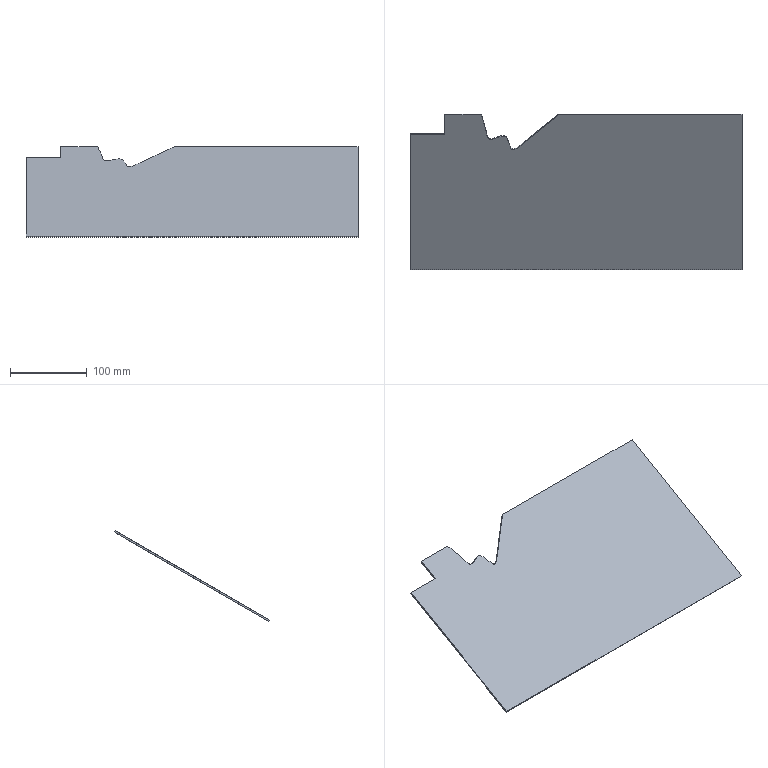Part | NX | features solid 2 | 1 solid | 11 faces | box 433.5 x 203.038 x 118.379 mm | volume 193522 mm3 | plane 9 | spline 2
STEP:
#1=CARTESIAN_POINT('',(-502.5,-191.,-72.946));
#2=VERTEX_POINT('',#1);
#3=CARTESIAN_POINT('',(-457.422,-191.,-72.946));
#4=VERTEX_POINT('',#3);
#5=CARTESIAN_POINT('',(-415.478,-191.,-72.946));
#6=DIRECTION('',(-1.,0.,0.));
#7=VECTOR('',#6,1000.);
#8=LINE('',#5,#7);
#9=EDGE_CURVE('',#2,#4,#8,.F.);
#10=ORIENTED_EDGE('',*,*,#9,.T.);
#11=CARTESIAN_POINT('',(-457.422,-190.,-74.678));
#12=VERTEX_POINT('',#11);
#13=CARTESIAN_POINT('',(-457.422,-140.,-161.281));
#14=DIRECTION('',(0.,-0.5,0.866));
#15=VECTOR('',#14,1000.);
#16=LINE('',#13,#15);
#17=EDGE_CURVE('',#12,#4,#16,.T.);
#18=ORIENTED_EDGE('',*,*,#17,.F.);
#19=CARTESIAN_POINT('',(-502.5,-190.,-74.678));
#20=VERTEX_POINT('',#19);
#21=CARTESIAN_POINT('',(-370.,-190.,-74.678));
#22=DIRECTION('',(1.,0.,0.));
#23=VECTOR('',#22,1000.);
#24=LINE('',#21,#23);
#25=EDGE_CURVE('',#20,#12,#24,.T.);
#26=ORIENTED_EDGE('',*,*,#25,.F.);
#27=CARTESIAN_POINT('',(-502.5,-97.191,-235.428));
#28=DIRECTION('',(0.,-0.5,0.866));
#29=VECTOR('',#28,1000.);
#30=LINE('',#27,#29);
#31=EDGE_CURVE('',#20,#2,#30,.T.);
#32=ORIENTED_EDGE('',*,*,#31,.T.);
#33=EDGE_LOOP('',(#10,#18,#26,#32));
#34=FACE_BOUND('',#33,.T.);
#35=CARTESIAN_POINT('',(-415.478,-140.,-161.281));
#36=DIRECTION('',(0.,-0.866,-0.5));
#37=DIRECTION('',(0.,0.5,-0.866));
#38=AXIS2_PLACEMENT_3D('',#35,#36,#37);
#39=PLANE('',#38);
#40=ADVANCED_FACE('',(#34),#39,.F.);
#41=CARTESIAN_POINT('',(-502.5,-367.603,-174.908));
#42=VERTEX_POINT('',#41);
#43=CARTESIAN_POINT('',(-502.5,-115.381,-29.287));
#44=DIRECTION('',(0.,-0.866,-0.5));
#45=VECTOR('',#44,1000.);
#46=LINE('',#43,#45);
#47=EDGE_CURVE('',#2,#42,#46,.T.);
#48=ORIENTED_EDGE('',*,*,#47,.F.);
#49=ORIENTED_EDGE('',*,*,#31,.F.);
#50=CARTESIAN_POINT('',(-502.5,-366.603,-176.64));
#51=VERTEX_POINT('',#50);
#52=CARTESIAN_POINT('',(-502.5,-114.381,-31.019));
#53=DIRECTION('',(0.,-0.866,-0.5));
#54=VECTOR('',#53,1000.);
#55=LINE('',#52,#54);
#56=EDGE_CURVE('',#20,#51,#55,.T.);
#57=ORIENTED_EDGE('',*,*,#56,.T.);
#58=CARTESIAN_POINT('',(-502.5,-273.793,-337.39));
#59=DIRECTION('',(0.,-0.5,0.866));
#60=VECTOR('',#59,1000.);
#61=LINE('',#58,#60);
#62=EDGE_CURVE('',#51,#42,#61,.T.);
#63=ORIENTED_EDGE('',*,*,#62,.T.);
#64=EDGE_LOOP('',(#48,#49,#57,#63));
#65=FACE_BOUND('',#64,.T.);
#66=CARTESIAN_POINT('',(-502.5,198.,-65.));
#67=DIRECTION('',(-1.,0.,0.));
#68=DIRECTION('',(0.,0.,-1.));
#69=AXIS2_PLACEMENT_3D('',#66,#67,#68);
#70=PLANE('',#69);
#71=ADVANCED_FACE('',(#65),#70,.T.);
#72=CARTESIAN_POINT('',(-69.,-367.603,-174.908));
#73=VERTEX_POINT('',#72);
#74=CARTESIAN_POINT('',(-370.,-367.603,-174.908));
#75=DIRECTION('',(1.,0.,0.));
#76=VECTOR('',#75,1000.);
#77=LINE('',#74,#76);
#78=EDGE_CURVE('',#42,#73,#77,.T.);
#79=ORIENTED_EDGE('',*,*,#78,.F.);
#80=ORIENTED_EDGE('',*,*,#62,.F.);
#81=CARTESIAN_POINT('',(-69.,-366.603,-176.64));
#82=VERTEX_POINT('',#81);
#83=CARTESIAN_POINT('',(-370.,-366.603,-176.64));
#84=DIRECTION('',(1.,0.,0.));
#85=VECTOR('',#84,1000.);
#86=LINE('',#83,#85);
#87=EDGE_CURVE('',#51,#82,#86,.T.);
#88=ORIENTED_EDGE('',*,*,#87,.T.);
#89=CARTESIAN_POINT('',(-69.,-318.851,-259.348));
#90=DIRECTION('',(0.,-0.5,0.866));
#91=VECTOR('',#90,1000.);
#92=LINE('',#89,#91);
#93=EDGE_CURVE('',#82,#73,#92,.T.);
#94=ORIENTED_EDGE('',*,*,#93,.T.);
#95=EDGE_LOOP('',(#79,#80,#88,#94));
#96=FACE_BOUND('',#95,.T.);
#97=CARTESIAN_POINT('',(-370.,-316.603,-263.242));
#98=DIRECTION('',(0.,-0.866,-0.5));
#99=DIRECTION('',(0.,0.5,-0.866));
#100=AXIS2_PLACEMENT_3D('',#97,#98,#99);
#101=PLANE('',#100);
#102=ADVANCED_FACE('',(#96),#101,.T.);
#103=CARTESIAN_POINT('',(-69.,-165.577,-58.268));
#104=VERTEX_POINT('',#103);
#105=CARTESIAN_POINT('',(-69.,-115.381,-29.287));
#106=DIRECTION('',(0.,-0.866,-0.5));
#107=VECTOR('',#106,1000.);
#108=LINE('',#105,#107);
#109=EDGE_CURVE('',#104,#73,#108,.T.);
#110=ORIENTED_EDGE('',*,*,#109,.T.);
#111=ORIENTED_EDGE('',*,*,#93,.F.);
#112=CARTESIAN_POINT('',(-69.,-164.577,-60.));
#113=VERTEX_POINT('',#112);
#114=CARTESIAN_POINT('',(-69.,-12.661,27.708));
#115=DIRECTION('',(0.,0.866,0.5));
#116=VECTOR('',#115,1000.);
#117=LINE('',#114,#116);
#118=EDGE_CURVE('',#82,#113,#117,.T.);
#119=ORIENTED_EDGE('',*,*,#118,.T.);
#120=CARTESIAN_POINT('',(-69.,-114.577,-146.603));
#121=DIRECTION('',(0.,-0.5,0.866));
#122=VECTOR('',#121,1000.);
#123=LINE('',#120,#122);
#124=EDGE_CURVE('',#113,#104,#123,.T.);
#125=ORIENTED_EDGE('',*,*,#124,.T.);
#126=EDGE_LOOP('',(#110,#111,#119,#125));
#127=FACE_BOUND('',#126,.T.);
#128=CARTESIAN_POINT('',(-69.,-64.381,-117.622));
#129=DIRECTION('',(-1.,0.,0.));
#130=DIRECTION('',(0.,0.,1.));
#131=AXIS2_PLACEMENT_3D('',#128,#129,#130);
#132=PLANE('',#131);
#133=ADVANCED_FACE('',(#127),#132,.F.);
#134=CARTESIAN_POINT('',(-308.051,-165.577,-58.268));
#135=VERTEX_POINT('',#134);
#136=CARTESIAN_POINT('',(-690.,-165.577,-58.268));
#137=DIRECTION('',(1.,0.,0.));
#138=VECTOR('',#137,1000.);
#139=LINE('',#136,#138);
#140=EDGE_CURVE('',#135,#104,#139,.T.);
#141=ORIENTED_EDGE('',*,*,#140,.T.);
#142=ORIENTED_EDGE('',*,*,#124,.F.);
#143=CARTESIAN_POINT('',(-308.051,-164.577,-60.));
#144=VERTEX_POINT('',#143);
#145=CARTESIAN_POINT('',(-370.,-164.577,-60.));
#146=DIRECTION('',(1.,0.,0.));
#147=VECTOR('',#146,1000.);
#148=LINE('',#145,#147);
#149=EDGE_CURVE('',#144,#113,#148,.T.);
#150=ORIENTED_EDGE('',*,*,#149,.F.);
#151=CARTESIAN_POINT('',(-308.051,-165.577,-58.268));
#152=CARTESIAN_POINT('',(-308.051,-165.243,-58.845));
#153=CARTESIAN_POINT('',(-308.051,-164.91,-59.423));
#154=CARTESIAN_POINT('',(-308.051,-164.577,-60.));
#155=B_SPLINE_CURVE_WITH_KNOTS('',3,(#151,#152,#153,#154),.UNSPECIFIED.,.F.,.F.,(4,4),(0.,0.01961),.UNSPECIFIED.);
#156=EDGE_CURVE('',#144,#135,#155,.F.);
#157=ORIENTED_EDGE('',*,*,#156,.T.);
#158=EDGE_LOOP('',(#141,#142,#150,#157));
#159=FACE_BOUND('',#158,.T.);
#160=CARTESIAN_POINT('',(-690.,-114.577,-146.603));
#161=DIRECTION('',(0.,-0.866,-0.5));
#162=DIRECTION('',(0.,0.5,-0.866));
#163=AXIS2_PLACEMENT_3D('',#160,#161,#162);
#164=PLANE('',#163);
#165=ADVANCED_FACE('',(#159),#164,.F.);
#166=CARTESIAN_POINT('',(-406.591,-174.699,-63.535));
#167=VERTEX_POINT('',#166);
#168=CARTESIAN_POINT('',(-308.051,-165.577,-58.268));
#169=CARTESIAN_POINT('',(-308.254,-165.738,-58.361));
#170=CARTESIAN_POINT('',(-309.078,-166.393,-58.739));
#171=CARTESIAN_POINT('',(-311.573,-168.377,-59.885));
#172=CARTESIAN_POINT('',(-314.699,-170.864,-61.32));
#173=CARTESIAN_POINT('',(-317.438,-173.043,-62.578));
#174=CARTESIAN_POINT('',(-319.159,-174.412,-63.369));
#175=CARTESIAN_POINT('',(-320.531,-175.504,-63.999));
#176=CARTESIAN_POINT('',(-321.734,-176.46,-64.552));
#177=CARTESIAN_POINT('',(-322.749,-177.268,-65.018));
#178=CARTESIAN_POINT('',(-323.368,-177.761,-65.302));
#179=CARTESIAN_POINT('',(-323.945,-178.22,-65.567));
#180=CARTESIAN_POINT('',(-324.267,-178.476,-65.715));
#181=CARTESIAN_POINT('',(-324.866,-178.952,-65.99));
#182=CARTESIAN_POINT('',(-326.005,-179.857,-66.513));
#183=CARTESIAN_POINT('',(-327.565,-181.096,-67.228));
#184=CARTESIAN_POINT('',(-329.008,-182.241,-67.889));
#185=CARTESIAN_POINT('',(-330.099,-183.104,-68.388));
#186=CARTESIAN_POINT('',(-330.751,-183.62,-68.685));
#187=CARTESIAN_POINT('',(-331.26,-184.023,-68.918));
#188=CARTESIAN_POINT('',(-331.563,-184.262,-69.056));
#189=CARTESIAN_POINT('',(-331.789,-184.44,-69.159));
#190=CARTESIAN_POINT('',(-331.889,-184.519,-69.204));
#191=CARTESIAN_POINT('',(-332.094,-184.681,-69.298));
#192=CARTESIAN_POINT('',(-332.422,-184.94,-69.447));
#193=CARTESIAN_POINT('',(-332.892,-185.311,-69.662));
#194=CARTESIAN_POINT('',(-333.473,-185.77,-69.927));
#195=CARTESIAN_POINT('',(-334.35,-186.462,-70.326));
#196=CARTESIAN_POINT('',(-335.768,-187.582,-70.972));
#197=CARTESIAN_POINT('',(-337.113,-188.645,-71.586));
#198=CARTESIAN_POINT('',(-338.186,-189.494,-72.076));
#199=CARTESIAN_POINT('',(-338.854,-190.023,-72.382));
#200=CARTESIAN_POINT('',(-339.296,-190.374,-72.584));
#201=CARTESIAN_POINT('',(-339.583,-190.601,-72.716));
#202=CARTESIAN_POINT('',(-339.731,-190.719,-72.784));
#203=CARTESIAN_POINT('',(-339.826,-190.794,-72.827));
#204=CARTESIAN_POINT('',(-339.867,-190.827,-72.846));
#205=CARTESIAN_POINT('',(-339.91,-190.862,-72.866));
#206=CARTESIAN_POINT('',(-339.899,-190.853,-72.861));
#207=CARTESIAN_POINT('',(-340.053,-190.976,-72.932));
#208=CARTESIAN_POINT('',(-340.29,-191.165,-73.041));
#209=CARTESIAN_POINT('',(-340.771,-191.55,-73.264));
#210=CARTESIAN_POINT('',(-341.409,-192.061,-73.558));
#211=CARTESIAN_POINT('',(-342.355,-192.817,-73.995));
#212=CARTESIAN_POINT('',(-343.384,-193.639,-74.47));
#213=CARTESIAN_POINT('',(-344.705,-194.696,-75.08));
#214=CARTESIAN_POINT('',(-345.431,-195.276,-75.415));
#215=CARTESIAN_POINT('',(-345.755,-195.535,-75.564));
#216=CARTESIAN_POINT('',(-345.829,-195.594,-75.598));
#217=CARTESIAN_POINT('',(-345.874,-195.63,-75.619));
#218=CARTESIAN_POINT('',(-345.862,-195.62,-75.614));
#219=CARTESIAN_POINT('',(-345.958,-195.696,-75.658));
#220=CARTESIAN_POINT('',(-346.164,-195.859,-75.751));
#221=CARTESIAN_POINT('',(-346.446,-196.081,-75.88));
#222=CARTESIAN_POINT('',(-346.815,-196.372,-76.048));
#223=CARTESIAN_POINT('',(-347.396,-196.83,-76.312));
#224=CARTESIAN_POINT('',(-348.418,-197.633,-76.776));
#225=CARTESIAN_POINT('',(-349.59,-198.549,-77.305));
#226=CARTESIAN_POINT('',(-350.61,-199.343,-77.763));
#227=CARTESIAN_POINT('',(-351.206,-199.806,-78.03));
#228=CARTESIAN_POINT('',(-351.55,-200.073,-78.184));
#229=CARTESIAN_POINT('',(-351.892,-200.337,-78.337));
#230=CARTESIAN_POINT('',(-351.989,-200.413,-78.381));
#231=CARTESIAN_POINT('',(-352.241,-200.61,-78.494));
#232=CARTESIAN_POINT('',(-352.844,-201.087,-78.77));
#233=CARTESIAN_POINT('',(-354.121,-202.108,-79.359));
#234=CARTESIAN_POINT('',(-355.859,-203.508,-80.167));
#235=CARTESIAN_POINT('',(-357.662,-204.965,-81.009));
#236=CARTESIAN_POINT('',(-358.887,-205.956,-81.581));
#237=CARTESIAN_POINT('',(-359.831,-206.715,-82.019));
#238=CARTESIAN_POINT('',(-360.359,-207.136,-82.262));
#239=CARTESIAN_POINT('',(-360.659,-207.374,-82.4));
#240=CARTESIAN_POINT('',(-360.752,-207.447,-82.442));
#241=CARTESIAN_POINT('',(-360.996,-207.639,-82.552));
#242=CARTESIAN_POINT('',(-361.347,-207.911,-82.709));
#243=CARTESIAN_POINT('',(-361.761,-208.225,-82.891));
#244=CARTESIAN_POINT('',(-362.402,-208.697,-83.164));
#245=CARTESIAN_POINT('',(-362.987,-209.108,-83.401));
#246=CARTESIAN_POINT('',(-363.56,-209.484,-83.618));
#247=CARTESIAN_POINT('',(-363.884,-209.689,-83.736));
#248=CARTESIAN_POINT('',(-364.508,-210.056,-83.948));
#249=CARTESIAN_POINT('',(-365.012,-210.321,-84.101));
#250=CARTESIAN_POINT('',(-365.536,-210.563,-84.241));
#251=CARTESIAN_POINT('',(-365.94,-210.729,-84.337));
#252=CARTESIAN_POINT('',(-366.646,-210.951,-84.465));
#253=CARTESIAN_POINT('',(-367.425,-211.082,-84.54));
#254=CARTESIAN_POINT('',(-368.333,-211.056,-84.525));
#255=CARTESIAN_POINT('',(-369.175,-210.699,-84.319));
#256=CARTESIAN_POINT('',(-369.765,-210.252,-84.061));
#257=CARTESIAN_POINT('',(-370.231,-209.75,-83.771));
#258=CARTESIAN_POINT('',(-370.469,-209.425,-83.584));
#259=CARTESIAN_POINT('',(-370.765,-208.98,-83.327));
#260=CARTESIAN_POINT('',(-371.03,-208.518,-83.06));
#261=CARTESIAN_POINT('',(-371.328,-207.923,-82.716));
#262=CARTESIAN_POINT('',(-371.493,-207.552,-82.502));
#263=CARTESIAN_POINT('',(-371.694,-207.072,-82.225));
#264=CARTESIAN_POINT('',(-371.857,-206.643,-81.978));
#265=CARTESIAN_POINT('',(-371.981,-206.302,-81.78));
#266=CARTESIAN_POINT('',(-372.097,-205.967,-81.587));
#267=CARTESIAN_POINT('',(-372.125,-205.885,-81.54));
#268=CARTESIAN_POINT('',(-372.208,-205.636,-81.396));
#269=CARTESIAN_POINT('',(-372.324,-205.28,-81.19));
#270=CARTESIAN_POINT('',(-372.501,-204.73,-80.873));
#271=CARTESIAN_POINT('',(-372.805,-203.771,-80.319));
#272=CARTESIAN_POINT('',(-373.133,-202.746,-79.727));
#273=CARTESIAN_POINT('',(-373.491,-201.665,-79.104));
#274=CARTESIAN_POINT('',(-373.753,-200.907,-78.666));
#275=CARTESIAN_POINT('',(-373.91,-200.471,-78.414));
#276=CARTESIAN_POINT('',(-374.005,-200.214,-78.266));
#277=CARTESIAN_POINT('',(-374.041,-200.116,-78.209));
#278=CARTESIAN_POINT('',(-374.198,-199.709,-77.974));
#279=CARTESIAN_POINT('',(-374.37,-199.289,-77.732));
#280=CARTESIAN_POINT('',(-374.697,-198.534,-77.296));
#281=CARTESIAN_POINT('',(-375.179,-197.571,-76.74));
#282=CARTESIAN_POINT('',(-375.8,-196.546,-76.148));
#283=CARTESIAN_POINT('',(-376.679,-195.372,-75.47));
#284=CARTESIAN_POINT('',(-377.626,-194.484,-74.958));
#285=CARTESIAN_POINT('',(-378.676,-193.875,-74.606));
#286=CARTESIAN_POINT('',(-379.431,-193.577,-74.434));
#287=CARTESIAN_POINT('',(-380.497,-193.358,-74.308));
#288=CARTESIAN_POINT('',(-381.613,-193.318,-74.284));
#289=CARTESIAN_POINT('',(-382.632,-193.409,-74.337));
#290=CARTESIAN_POINT('',(-383.405,-193.546,-74.416));
#291=CARTESIAN_POINT('',(-383.833,-193.637,-74.469));
#292=CARTESIAN_POINT('',(-384.236,-193.735,-74.525));
#293=CARTESIAN_POINT('',(-384.354,-193.767,-74.544));
#294=CARTESIAN_POINT('',(-384.633,-193.843,-74.588));
#295=CARTESIAN_POINT('',(-385.117,-193.986,-74.67));
#296=CARTESIAN_POINT('',(-386.299,-194.367,-74.89));
#297=CARTESIAN_POINT('',(-388.071,-195.014,-75.264));
#298=CARTESIAN_POINT('',(-390.198,-195.816,-75.727));
#299=CARTESIAN_POINT('',(-391.407,-196.255,-75.98));
#300=CARTESIAN_POINT('',(-392.231,-196.542,-76.146));
#301=CARTESIAN_POINT('',(-392.665,-196.686,-76.229));
#302=CARTESIAN_POINT('',(-392.914,-196.765,-76.274));
#303=CARTESIAN_POINT('',(-392.99,-196.789,-76.288));
#304=CARTESIAN_POINT('',(-393.407,-196.911,-76.359));
#305=CARTESIAN_POINT('',(-393.833,-197.025,-76.425));
#306=CARTESIAN_POINT('',(-394.611,-197.212,-76.533));
#307=CARTESIAN_POINT('',(-395.626,-197.383,-76.632));
#308=CARTESIAN_POINT('',(-396.547,-197.445,-76.667));
#309=CARTESIAN_POINT('',(-397.253,-197.42,-76.652));
#310=CARTESIAN_POINT('',(-397.683,-197.38,-76.63));
#311=CARTESIAN_POINT('',(-398.358,-197.252,-76.555));
#312=CARTESIAN_POINT('',(-399.085,-197.013,-76.417));
#313=CARTESIAN_POINT('',(-399.923,-196.538,-76.144));
#314=CARTESIAN_POINT('',(-400.501,-195.946,-75.802));
#315=CARTESIAN_POINT('',(-400.934,-195.365,-75.466));
#316=CARTESIAN_POINT('',(-401.27,-194.783,-75.13));
#317=CARTESIAN_POINT('',(-401.416,-194.48,-74.955));
#318=CARTESIAN_POINT('',(-401.666,-193.917,-74.63));
#319=CARTESIAN_POINT('',(-401.937,-193.158,-74.192));
#320=CARTESIAN_POINT('',(-402.192,-192.271,-73.68));
#321=CARTESIAN_POINT('',(-402.359,-191.576,-73.278));
#322=CARTESIAN_POINT('',(-402.446,-191.182,-73.051));
#323=CARTESIAN_POINT('',(-402.522,-190.815,-72.839));
#324=CARTESIAN_POINT('',(-402.549,-190.678,-72.76));
#325=CARTESIAN_POINT('',(-402.606,-190.384,-72.59));
#326=CARTESIAN_POINT('',(-402.706,-189.844,-72.279));
#327=CARTESIAN_POINT('',(-402.842,-189.052,-71.821));
#328=CARTESIAN_POINT('',(-402.997,-188.128,-71.288));
#329=CARTESIAN_POINT('',(-403.092,-187.575,-70.968));
#330=CARTESIAN_POINT('',(-403.157,-187.194,-70.749));
#331=CARTESIAN_POINT('',(-403.205,-186.92,-70.59));
#332=CARTESIAN_POINT('',(-403.227,-186.796,-70.519));
#333=CARTESIAN_POINT('',(-403.285,-186.475,-70.333));
#334=CARTESIAN_POINT('',(-403.35,-186.12,-70.129));
#335=CARTESIAN_POINT('',(-403.473,-185.48,-69.759));
#336=CARTESIAN_POINT('',(-403.65,-184.615,-69.26));
#337=CARTESIAN_POINT('',(-403.873,-183.626,-68.688));
#338=CARTESIAN_POINT('',(-404.106,-182.688,-68.147));
#339=CARTESIAN_POINT('',(-404.342,-181.82,-67.646));
#340=CARTESIAN_POINT('',(-404.626,-180.842,-67.081));
#341=CARTESIAN_POINT('',(-404.889,-179.989,-66.589));
#342=CARTESIAN_POINT('',(-405.126,-179.246,-66.16));
#343=CARTESIAN_POINT('',(-405.292,-178.738,-65.867));
#344=CARTESIAN_POINT('',(-405.55,-177.956,-65.415));
#345=CARTESIAN_POINT('',(-405.826,-177.112,-64.928));
#346=CARTESIAN_POINT('',(-406.254,-175.791,-64.165));
#347=CARTESIAN_POINT('',(-406.489,-175.042,-63.732));
#348=CARTESIAN_POINT('',(-406.591,-174.699,-63.535));
#349=B_SPLINE_CURVE_WITH_KNOTS('',3,(#168,#169,#170,#171,#172,#173,#174,#175,#176,#177,#178,#179,#180,#181,#182,#183,#184,#185,#186,#187,#188,#189,#190,#191,#192,#193,#194,#195,#196,#197,#198,#199,#200,#201,#202,#203,#204,#205,#206,#207,#208,#209,#210,#211,#212,#213,#214,#215,#216,#217,#218,#219,#220,#221,#222,#223,#224,#225,#226,#227,#228,#229,#230,#231,#232,#233,#234,#235,#236,#237,#238,#239,#240,#241,#242,#243,#244,#245,#246,#247,#248,#249,#250,#251,#252,#253,#254,#255,#256,#257,#258,#259,#260,#261,#262,#263,#264,#265,#266,#267,#268,#269,#270,#271,#272,#273,#274,#275,#276,#277,#278,#279,#280,#281,#282,#283,#284,#285,#286,#287,#288,#289,#290,#291,#292,#293,#294,#295,#296,#297,#298,#299,#300,#301,#302,#303,#304,#305,#306,#307,#308,#309,#310,#311,#312,#313,#314,#315,#316,#317,#318,#319,#320,#321,#322,#323,#324,#325,#326,#327,#328,#329,#330,#331,#332,#333,#334,#335,#336,#337,#338,#339,#340,#341,#342,#343,#344,#345,#346,#347,#348),.UNSPECIFIED.,.F.,.F.,(4,1,1,1,1,1,1,1,1,1,1,1,1,1,1,1,1,1,1,1,1,1,1,1,1,1,1,1,1,1,1,1,1,1,1,1,1,1,1,1,1,1,1,1,1,1,1,1,1,1,1,1,1,1,1,1,1,1,1,1,1,1,1,1,1,1,1,1,1,1,1,1,1,1,1,1,1,1,1,1,1,1,1,1,1,1,1,1,1,1,1,1,1,1,1,1,1,1,1,1,1,1,1,1,1,1,1,1,1,1,1,1,1,1,1,1,1,1,1,1,1,1,1,1,1,1,1,1,1,1,1,1,1,1,1,1,1,1,1,1,1,1,1,1,1,1,1,1,1,1,1,1,1,1,1,1,1,1,1,1,1,1,1,1,1,1,1,1,1,1,1,1,1,1,1,1,1,1,4),(0.,0.03125,0.0625,0.09375,0.1094,0.1172,0.125,0.1328,0.1367,0.1406,0.1426,0.1445,0.1484,0.1562,0.1719,0.1875,0.1953,0.2031,0.207,0.2109,0.2129,0.2139,0.2148,0.2168,0.2188,0.2227,0.2266,0.2344,0.25,0.2578,0.2656,0.2734,0.2773,0.2812,0.2832,0.2842,0.2852,0.2856,0.2861,0.2871,0.2891,0.293,0.2969,0.3047,0.3125,0.3281,0.332,0.3359,0.3379,0.3389,0.3398,0.3418,0.3438,0.3477,0.3516,0.3594,0.375,0.3828,0.3867,0.3906,0.3926,0.3945,0.3984,0.4062,0.4219,0.4375,0.4453,0.4531,0.4609,0.4688,0.4707,0.4727,0.4746,0.4766,0.4805,0.4844,0.4922,0.4961,0.5,0.5039,0.5078,0.5117,0.5156,0.5195,0.5234,0.5312,0.5391,0.543,0.5469,0.5508,0.5547,0.5586,0.5625,0.5664,0.5703,0.5742,0.5762,0.5781,0.5801,0.582,0.5859,0.5898,0.5938,0.6016,0.6094,0.6172,0.6211,0.623,0.625,0.627,0.6289,0.6328,0.6406,0.6484,0.6562,0.6719,0.6797,0.6875,0.6953,0.7031,0.7109,0.7148,0.7168,0.7188,0.7207,0.7227,0.7266,0.7344,0.75,0.7578,0.7656,0.7734,0.7773,0.7793,0.7812,0.7832,0.7852,0.7891,0.7969,0.8047,0.8086,0.8125,0.8164,0.8203,0.8281,0.8359,0.8398,0.8438,0.8477,0.8516,0.8594,0.8672,0.8711,0.873,0.875,0.877,0.8789,0.8828,0.8906,0.8945,0.8984,0.9023,0.9043,0.9062,0.9082,0.9102,0.9141,0.9219,0.9297,0.9375,0.9453,0.9531,0.9609,0.9648,0.9688,0.9727,0.9766,0.9844,1.),.UNSPECIFIED.);
#350=EDGE_CURVE('',#167,#135,#349,.F.);
#351=ORIENTED_EDGE('',*,*,#350,.T.);
#352=ORIENTED_EDGE('',*,*,#156,.F.);
#353=CARTESIAN_POINT('',(-406.591,-173.699,-65.267));
#354=VERTEX_POINT('',#353);
#355=CARTESIAN_POINT('',(-406.591,-173.699,-65.267));
#356=CARTESIAN_POINT('',(-406.198,-175.018,-66.028));
#357=CARTESIAN_POINT('',(-405.31,-177.635,-67.539));
#358=CARTESIAN_POINT('',(-404.07,-181.579,-69.816));
#359=CARTESIAN_POINT('',(-403.218,-185.599,-72.137));
#360=CARTESIAN_POINT('',(-402.724,-188.984,-74.092));
#361=CARTESIAN_POINT('',(-402.116,-191.664,-75.639));
#362=CARTESIAN_POINT('',(-401.443,-193.608,-76.761));
#363=CARTESIAN_POINT('',(-400.277,-195.451,-77.825));
#364=CARTESIAN_POINT('',(-398.119,-196.479,-78.419));
#365=CARTESIAN_POINT('',(-395.713,-196.453,-78.404));
#366=CARTESIAN_POINT('',(-393.422,-195.965,-78.122));
#367=CARTESIAN_POINT('',(-391.237,-195.199,-77.68));
#368=CARTESIAN_POINT('',(-389.076,-194.396,-77.216));
#369=CARTESIAN_POINT('',(-386.916,-193.585,-76.748));
#370=CARTESIAN_POINT('',(-384.735,-192.829,-76.311));
#371=CARTESIAN_POINT('',(-382.478,-192.321,-76.018));
#372=CARTESIAN_POINT('',(-380.027,-192.293,-76.002));
#373=CARTESIAN_POINT('',(-377.81,-193.228,-76.542));
#374=CARTESIAN_POINT('',(-376.246,-194.838,-77.471));
#375=CARTESIAN_POINT('',(-375.094,-196.659,-78.523));
#376=CARTESIAN_POINT('',(-373.938,-199.203,-79.991));
#377=CARTESIAN_POINT('',(-373.091,-201.861,-81.526));
#378=CARTESIAN_POINT('',(-372.258,-204.517,-83.06));
#379=CARTESIAN_POINT('',(-371.569,-206.489,-84.198));
#380=CARTESIAN_POINT('',(-370.763,-208.085,-85.12));
#381=CARTESIAN_POINT('',(-369.85,-209.221,-85.775));
#382=CARTESIAN_POINT('',(-368.903,-209.888,-86.16));
#383=CARTESIAN_POINT('',(-367.701,-210.131,-86.301));
#384=CARTESIAN_POINT('',(-366.103,-209.875,-86.153));
#385=CARTESIAN_POINT('',(-364.359,-209.024,-85.662));
#386=CARTESIAN_POINT('',(-362.466,-207.771,-84.938));
#387=CARTESIAN_POINT('',(-360.088,-205.946,-83.884));
#388=CARTESIAN_POINT('',(-357.201,-203.588,-82.523));
#389=CARTESIAN_POINT('',(-353.721,-200.772,-80.897));
#390=CARTESIAN_POINT('',(-350.184,-198.011,-79.303));
#391=CARTESIAN_POINT('',(-346.645,-195.251,-77.71));
#392=CARTESIAN_POINT('',(-341.984,-191.516,-75.553));
#393=CARTESIAN_POINT('',(-336.139,-186.866,-72.869));
#394=CARTESIAN_POINT('',(-329.092,-181.318,-69.665));
#395=CARTESIAN_POINT('',(-322.081,-175.735,-66.442));
#396=CARTESIAN_POINT('',(-315.065,-170.157,-63.221));
#397=CARTESIAN_POINT('',(-310.391,-166.435,-61.073));
#398=CARTESIAN_POINT('',(-308.051,-164.577,-60.));
#399=B_SPLINE_CURVE_WITH_KNOTS('',3,(#355,#356,#357,#358,#359,#360,#361,#362,#363,#364,#365,#366,#367,#368,#369,#370,#371,#372,#373,#374,#375,#376,#377,#378,#379,#380,#381,#382,#383,#384,#385,#386,#387,#388,#389,#390,#391,#392,#393,#394,#395,#396,#397,#398),.UNSPECIFIED.,.F.,.F.,(4,1,1,1,1,1,1,1,1,1,1,1,1,1,1,1,1,1,1,1,1,1,1,1,1,1,1,1,1,1,1,1,1,1,1,1,1,1,1,1,1,4),(0.,0.004714,0.009429,0.01414,0.01886,0.02121,0.02357,0.02593,0.02829,0.03064,0.033,0.03536,0.03771,0.04007,0.04243,0.04479,0.04714,0.0495,0.05186,0.05422,0.05657,0.06129,0.06364,0.066,0.06836,0.06954,0.07072,0.07189,0.07307,0.07543,0.07779,0.08014,0.08486,0.08957,0.09429,0.099,0.1037,0.1131,0.1226,0.132,0.1414,0.1509),.UNSPECIFIED.);
#400=EDGE_CURVE('',#354,#144,#399,.T.);
#401=ORIENTED_EDGE('',*,*,#400,.F.);
#402=CARTESIAN_POINT('',(-406.591,-174.699,-63.535));
#403=CARTESIAN_POINT('',(-406.591,-174.366,-64.112));
#404=CARTESIAN_POINT('',(-406.591,-174.033,-64.689));
#405=CARTESIAN_POINT('',(-406.591,-173.699,-65.267));
#406=B_SPLINE_CURVE_WITH_KNOTS('',3,(#402,#403,#404,#405),.UNSPECIFIED.,.F.,.F.,(4,4),(0.,0.01961),.UNSPECIFIED.);
#407=EDGE_CURVE('',#354,#167,#406,.F.);
#408=ORIENTED_EDGE('',*,*,#407,.T.);
#409=EDGE_LOOP('',(#351,#352,#401,#408));
#410=FACE_BOUND('',#409,.T.);
#411=CARTESIAN_POINT('',(-308.051,-164.577,-60.));
#412=CARTESIAN_POINT('',(-308.051,-165.577,-58.268));
#413=CARTESIAN_POINT('',(-308.254,-164.738,-60.093));
#414=CARTESIAN_POINT('',(-308.254,-165.738,-58.361));
#415=CARTESIAN_POINT('',(-309.078,-165.393,-60.471));
#416=CARTESIAN_POINT('',(-309.078,-166.393,-58.739));
#417=CARTESIAN_POINT('',(-311.573,-167.377,-61.617));
#418=CARTESIAN_POINT('',(-311.573,-168.377,-59.885));
#419=CARTESIAN_POINT('',(-314.699,-169.864,-63.052));
#420=CARTESIAN_POINT('',(-314.699,-170.864,-61.32));
#421=CARTESIAN_POINT('',(-317.438,-172.043,-64.31));
#422=CARTESIAN_POINT('',(-317.438,-173.043,-62.578));
#423=CARTESIAN_POINT('',(-319.159,-173.412,-65.101));
#424=CARTESIAN_POINT('',(-319.159,-174.412,-63.369));
#425=CARTESIAN_POINT('',(-320.531,-174.504,-65.731));
#426=CARTESIAN_POINT('',(-320.531,-175.504,-63.999));
#427=CARTESIAN_POINT('',(-321.734,-175.46,-66.284));
#428=CARTESIAN_POINT('',(-321.734,-176.46,-64.552));
#429=CARTESIAN_POINT('',(-322.749,-176.268,-66.75));
#430=CARTESIAN_POINT('',(-322.749,-177.268,-65.018));
#431=CARTESIAN_POINT('',(-323.368,-176.761,-67.034));
#432=CARTESIAN_POINT('',(-323.368,-177.761,-65.302));
#433=CARTESIAN_POINT('',(-323.945,-177.22,-67.299));
#434=CARTESIAN_POINT('',(-323.945,-178.22,-65.567));
#435=CARTESIAN_POINT('',(-324.267,-177.476,-67.447));
#436=CARTESIAN_POINT('',(-324.267,-178.476,-65.715));
#437=CARTESIAN_POINT('',(-324.866,-177.952,-67.722));
#438=CARTESIAN_POINT('',(-324.866,-178.952,-65.99));
#439=CARTESIAN_POINT('',(-326.005,-178.857,-68.245));
#440=CARTESIAN_POINT('',(-326.005,-179.857,-66.513));
#441=CARTESIAN_POINT('',(-327.565,-180.096,-68.96));
#442=CARTESIAN_POINT('',(-327.565,-181.096,-67.228));
#443=CARTESIAN_POINT('',(-329.008,-181.241,-69.621));
#444=CARTESIAN_POINT('',(-329.008,-182.241,-67.889));
#445=CARTESIAN_POINT('',(-330.099,-182.104,-70.12));
#446=CARTESIAN_POINT('',(-330.099,-183.104,-68.388));
#447=CARTESIAN_POINT('',(-330.751,-182.62,-70.417));
#448=CARTESIAN_POINT('',(-330.751,-183.62,-68.685));
#449=CARTESIAN_POINT('',(-331.26,-183.023,-70.65));
#450=CARTESIAN_POINT('',(-331.26,-184.023,-68.918));
#451=CARTESIAN_POINT('',(-331.563,-183.262,-70.788));
#452=CARTESIAN_POINT('',(-331.563,-184.262,-69.056));
#453=CARTESIAN_POINT('',(-331.789,-183.44,-70.891));
#454=CARTESIAN_POINT('',(-331.789,-184.44,-69.159));
#455=CARTESIAN_POINT('',(-331.889,-183.519,-70.936));
#456=CARTESIAN_POINT('',(-331.889,-184.519,-69.204));
#457=CARTESIAN_POINT('',(-332.094,-183.681,-71.03));
#458=CARTESIAN_POINT('',(-332.094,-184.681,-69.298));
#459=CARTESIAN_POINT('',(-332.422,-183.94,-71.179));
#460=CARTESIAN_POINT('',(-332.422,-184.94,-69.447));
#461=CARTESIAN_POINT('',(-332.892,-184.311,-71.394));
#462=CARTESIAN_POINT('',(-332.892,-185.311,-69.662));
#463=CARTESIAN_POINT('',(-333.473,-184.77,-71.659));
#464=CARTESIAN_POINT('',(-333.473,-185.77,-69.927));
#465=CARTESIAN_POINT('',(-334.35,-185.462,-72.058));
#466=CARTESIAN_POINT('',(-334.35,-186.462,-70.326));
#467=CARTESIAN_POINT('',(-335.768,-186.582,-72.705));
#468=CARTESIAN_POINT('',(-335.768,-187.582,-70.972));
#469=CARTESIAN_POINT('',(-337.113,-187.645,-73.318));
#470=CARTESIAN_POINT('',(-337.113,-188.645,-71.586));
#471=CARTESIAN_POINT('',(-338.186,-188.494,-73.808));
#472=CARTESIAN_POINT('',(-338.186,-189.494,-72.076));
#473=CARTESIAN_POINT('',(-338.854,-189.023,-74.114));
#474=CARTESIAN_POINT('',(-338.854,-190.023,-72.382));
#475=CARTESIAN_POINT('',(-339.296,-189.374,-74.316));
#476=CARTESIAN_POINT('',(-339.296,-190.374,-72.584));
#477=CARTESIAN_POINT('',(-339.583,-189.601,-74.448));
#478=CARTESIAN_POINT('',(-339.583,-190.601,-72.716));
#479=CARTESIAN_POINT('',(-339.731,-189.719,-74.516));
#480=CARTESIAN_POINT('',(-339.731,-190.719,-72.784));
#481=CARTESIAN_POINT('',(-339.826,-189.794,-74.559));
#482=CARTESIAN_POINT('',(-339.826,-190.794,-72.827));
#483=CARTESIAN_POINT('',(-339.867,-189.827,-74.578));
#484=CARTESIAN_POINT('',(-339.867,-190.827,-72.846));
#485=CARTESIAN_POINT('',(-339.91,-189.862,-74.598));
#486=CARTESIAN_POINT('',(-339.91,-190.862,-72.866));
#487=CARTESIAN_POINT('',(-339.899,-189.853,-74.593));
#488=CARTESIAN_POINT('',(-339.899,-190.853,-72.861));
#489=CARTESIAN_POINT('',(-340.053,-189.976,-74.664));
#490=CARTESIAN_POINT('',(-340.053,-190.976,-72.932));
#491=CARTESIAN_POINT('',(-340.29,-190.165,-74.774));
#492=CARTESIAN_POINT('',(-340.29,-191.165,-73.041));
#493=CARTESIAN_POINT('',(-340.771,-190.55,-74.996));
#494=CARTESIAN_POINT('',(-340.771,-191.55,-73.264));
#495=CARTESIAN_POINT('',(-341.409,-191.061,-75.29));
#496=CARTESIAN_POINT('',(-341.409,-192.061,-73.558));
#497=CARTESIAN_POINT('',(-342.355,-191.817,-75.727));
#498=CARTESIAN_POINT('',(-342.355,-192.817,-73.995));
#499=CARTESIAN_POINT('',(-343.384,-192.639,-76.202));
#500=CARTESIAN_POINT('',(-343.384,-193.639,-74.47));
#501=CARTESIAN_POINT('',(-344.705,-193.696,-76.812));
#502=CARTESIAN_POINT('',(-344.705,-194.696,-75.08));
#503=CARTESIAN_POINT('',(-345.431,-194.276,-77.147));
#504=CARTESIAN_POINT('',(-345.431,-195.276,-75.415));
#505=CARTESIAN_POINT('',(-345.755,-194.535,-77.296));
#506=CARTESIAN_POINT('',(-345.755,-195.535,-75.564));
#507=CARTESIAN_POINT('',(-345.829,-194.594,-77.331));
#508=CARTESIAN_POINT('',(-345.829,-195.594,-75.598));
#509=CARTESIAN_POINT('',(-345.874,-194.63,-77.351));
#510=CARTESIAN_POINT('',(-345.874,-195.63,-75.619));
#511=CARTESIAN_POINT('',(-345.862,-194.62,-77.346));
#512=CARTESIAN_POINT('',(-345.862,-195.62,-75.614));
#513=CARTESIAN_POINT('',(-345.958,-194.696,-77.39));
#514=CARTESIAN_POINT('',(-345.958,-195.696,-75.658));
#515=CARTESIAN_POINT('',(-346.164,-194.859,-77.483));
#516=CARTESIAN_POINT('',(-346.164,-195.859,-75.751));
#517=CARTESIAN_POINT('',(-346.446,-195.081,-77.612));
#518=CARTESIAN_POINT('',(-346.446,-196.081,-75.88));
#519=CARTESIAN_POINT('',(-346.815,-195.372,-77.78));
#520=CARTESIAN_POINT('',(-346.815,-196.372,-76.048));
#521=CARTESIAN_POINT('',(-347.396,-195.83,-78.044));
#522=CARTESIAN_POINT('',(-347.396,-196.83,-76.312));
#523=CARTESIAN_POINT('',(-348.418,-196.633,-78.508));
#524=CARTESIAN_POINT('',(-348.418,-197.633,-76.776));
#525=CARTESIAN_POINT('',(-349.59,-197.549,-79.037));
#526=CARTESIAN_POINT('',(-349.59,-198.549,-77.305));
#527=CARTESIAN_POINT('',(-350.61,-198.343,-79.495));
#528=CARTESIAN_POINT('',(-350.61,-199.343,-77.763));
#529=CARTESIAN_POINT('',(-351.206,-198.806,-79.762));
#530=CARTESIAN_POINT('',(-351.206,-199.806,-78.03));
#531=CARTESIAN_POINT('',(-351.55,-199.073,-79.916));
#532=CARTESIAN_POINT('',(-351.55,-200.073,-78.184));
#533=CARTESIAN_POINT('',(-351.892,-199.337,-80.069));
#534=CARTESIAN_POINT('',(-351.892,-200.337,-78.337));
#535=CARTESIAN_POINT('',(-351.989,-199.413,-80.113));
#536=CARTESIAN_POINT('',(-351.989,-200.413,-78.381));
#537=CARTESIAN_POINT('',(-352.241,-199.61,-80.226));
#538=CARTESIAN_POINT('',(-352.241,-200.61,-78.494));
#539=CARTESIAN_POINT('',(-352.844,-200.087,-80.502));
#540=CARTESIAN_POINT('',(-352.844,-201.087,-78.77));
#541=CARTESIAN_POINT('',(-354.121,-201.108,-81.091));
#542=CARTESIAN_POINT('',(-354.121,-202.108,-79.359));
#543=CARTESIAN_POINT('',(-355.859,-202.508,-81.899));
#544=CARTESIAN_POINT('',(-355.859,-203.508,-80.167));
#545=CARTESIAN_POINT('',(-357.662,-203.965,-82.741));
#546=CARTESIAN_POINT('',(-357.662,-204.965,-81.009));
#547=CARTESIAN_POINT('',(-358.887,-204.956,-83.313));
#548=CARTESIAN_POINT('',(-358.887,-205.956,-81.581));
#549=CARTESIAN_POINT('',(-359.831,-205.715,-83.751));
#550=CARTESIAN_POINT('',(-359.831,-206.715,-82.019));
#551=CARTESIAN_POINT('',(-360.359,-206.136,-83.994));
#552=CARTESIAN_POINT('',(-360.359,-207.136,-82.262));
#553=CARTESIAN_POINT('',(-360.659,-206.374,-84.132));
#554=CARTESIAN_POINT('',(-360.659,-207.374,-82.4));
#555=CARTESIAN_POINT('',(-360.752,-206.447,-84.174));
#556=CARTESIAN_POINT('',(-360.752,-207.447,-82.442));
#557=CARTESIAN_POINT('',(-360.996,-206.639,-84.284));
#558=CARTESIAN_POINT('',(-360.996,-207.639,-82.552));
#559=CARTESIAN_POINT('',(-361.347,-206.911,-84.441));
#560=CARTESIAN_POINT('',(-361.347,-207.911,-82.709));
#561=CARTESIAN_POINT('',(-361.761,-207.225,-84.623));
#562=CARTESIAN_POINT('',(-361.761,-208.225,-82.891));
#563=CARTESIAN_POINT('',(-362.402,-207.697,-84.896));
#564=CARTESIAN_POINT('',(-362.402,-208.697,-83.164));
#565=CARTESIAN_POINT('',(-362.987,-208.108,-85.133));
#566=CARTESIAN_POINT('',(-362.987,-209.108,-83.401));
#567=CARTESIAN_POINT('',(-363.56,-208.484,-85.35));
#568=CARTESIAN_POINT('',(-363.56,-209.484,-83.618));
#569=CARTESIAN_POINT('',(-363.884,-208.689,-85.468));
#570=CARTESIAN_POINT('',(-363.884,-209.689,-83.736));
#571=CARTESIAN_POINT('',(-364.508,-209.056,-85.68));
#572=CARTESIAN_POINT('',(-364.508,-210.056,-83.948));
#573=CARTESIAN_POINT('',(-365.012,-209.321,-85.833));
#574=CARTESIAN_POINT('',(-365.012,-210.321,-84.101));
#575=CARTESIAN_POINT('',(-365.536,-209.563,-85.973));
#576=CARTESIAN_POINT('',(-365.536,-210.563,-84.241));
#577=CARTESIAN_POINT('',(-365.94,-209.729,-86.069));
#578=CARTESIAN_POINT('',(-365.94,-210.729,-84.337));
#579=CARTESIAN_POINT('',(-366.646,-209.951,-86.197));
#580=CARTESIAN_POINT('',(-366.646,-210.951,-84.465));
#581=CARTESIAN_POINT('',(-367.425,-210.082,-86.272));
#582=CARTESIAN_POINT('',(-367.425,-211.082,-84.54));
#583=CARTESIAN_POINT('',(-368.333,-210.056,-86.257));
#584=CARTESIAN_POINT('',(-368.333,-211.056,-84.525));
#585=CARTESIAN_POINT('',(-369.175,-209.699,-86.051));
#586=CARTESIAN_POINT('',(-369.175,-210.699,-84.319));
#587=CARTESIAN_POINT('',(-369.765,-209.252,-85.793));
#588=CARTESIAN_POINT('',(-369.765,-210.252,-84.061));
#589=CARTESIAN_POINT('',(-370.231,-208.75,-85.503));
#590=CARTESIAN_POINT('',(-370.231,-209.75,-83.771));
#591=CARTESIAN_POINT('',(-370.469,-208.425,-85.316));
#592=CARTESIAN_POINT('',(-370.469,-209.425,-83.584));
#593=CARTESIAN_POINT('',(-370.765,-207.98,-85.059));
#594=CARTESIAN_POINT('',(-370.765,-208.98,-83.327));
#595=CARTESIAN_POINT('',(-371.03,-207.518,-84.792));
#596=CARTESIAN_POINT('',(-371.03,-208.518,-83.06));
#597=CARTESIAN_POINT('',(-371.328,-206.923,-84.449));
#598=CARTESIAN_POINT('',(-371.328,-207.923,-82.716));
#599=CARTESIAN_POINT('',(-371.493,-206.552,-84.234));
#600=CARTESIAN_POINT('',(-371.493,-207.552,-82.502));
#601=CARTESIAN_POINT('',(-371.694,-206.072,-83.957));
#602=CARTESIAN_POINT('',(-371.694,-207.072,-82.225));
#603=CARTESIAN_POINT('',(-371.857,-205.643,-83.71));
#604=CARTESIAN_POINT('',(-371.857,-206.643,-81.978));
#605=CARTESIAN_POINT('',(-371.981,-205.302,-83.513));
#606=CARTESIAN_POINT('',(-371.981,-206.302,-81.78));
#607=CARTESIAN_POINT('',(-372.097,-204.967,-83.319));
#608=CARTESIAN_POINT('',(-372.097,-205.967,-81.587));
#609=CARTESIAN_POINT('',(-372.125,-204.885,-83.272));
#610=CARTESIAN_POINT('',(-372.125,-205.885,-81.54));
#611=CARTESIAN_POINT('',(-372.208,-204.636,-83.128));
#612=CARTESIAN_POINT('',(-372.208,-205.636,-81.396));
#613=CARTESIAN_POINT('',(-372.324,-204.28,-82.922));
#614=CARTESIAN_POINT('',(-372.324,-205.28,-81.19));
#615=CARTESIAN_POINT('',(-372.501,-203.73,-82.605));
#616=CARTESIAN_POINT('',(-372.501,-204.73,-80.873));
#617=CARTESIAN_POINT('',(-372.805,-202.771,-82.051));
#618=CARTESIAN_POINT('',(-372.805,-203.771,-80.319));
#619=CARTESIAN_POINT('',(-373.133,-201.746,-81.459));
#620=CARTESIAN_POINT('',(-373.133,-202.746,-79.727));
#621=CARTESIAN_POINT('',(-373.491,-200.665,-80.836));
#622=CARTESIAN_POINT('',(-373.491,-201.665,-79.104));
#623=CARTESIAN_POINT('',(-373.753,-199.907,-80.398));
#624=CARTESIAN_POINT('',(-373.753,-200.907,-78.666));
#625=CARTESIAN_POINT('',(-373.91,-199.471,-80.146));
#626=CARTESIAN_POINT('',(-373.91,-200.471,-78.414));
#627=CARTESIAN_POINT('',(-374.005,-199.214,-79.998));
#628=CARTESIAN_POINT('',(-374.005,-200.214,-78.266));
#629=CARTESIAN_POINT('',(-374.041,-199.116,-79.941));
#630=CARTESIAN_POINT('',(-374.041,-200.116,-78.209));
#631=CARTESIAN_POINT('',(-374.198,-198.709,-79.706));
#632=CARTESIAN_POINT('',(-374.198,-199.709,-77.974));
#633=CARTESIAN_POINT('',(-374.37,-198.289,-79.464));
#634=CARTESIAN_POINT('',(-374.37,-199.289,-77.732));
#635=CARTESIAN_POINT('',(-374.697,-197.534,-79.028));
#636=CARTESIAN_POINT('',(-374.697,-198.534,-77.296));
#637=CARTESIAN_POINT('',(-375.179,-196.571,-78.472));
#638=CARTESIAN_POINT('',(-375.179,-197.571,-76.74));
#639=CARTESIAN_POINT('',(-375.8,-195.546,-77.88));
#640=CARTESIAN_POINT('',(-375.8,-196.546,-76.148));
#641=CARTESIAN_POINT('',(-376.679,-194.372,-77.202));
#642=CARTESIAN_POINT('',(-376.679,-195.372,-75.47));
#643=CARTESIAN_POINT('',(-377.626,-193.484,-76.69));
#644=CARTESIAN_POINT('',(-377.626,-194.484,-74.958));
#645=CARTESIAN_POINT('',(-378.676,-192.875,-76.338));
#646=CARTESIAN_POINT('',(-378.676,-193.875,-74.606));
#647=CARTESIAN_POINT('',(-379.431,-192.577,-76.166));
#648=CARTESIAN_POINT('',(-379.431,-193.577,-74.434));
#649=CARTESIAN_POINT('',(-380.497,-192.358,-76.04));
#650=CARTESIAN_POINT('',(-380.497,-193.358,-74.308));
#651=CARTESIAN_POINT('',(-381.613,-192.318,-76.017));
#652=CARTESIAN_POINT('',(-381.613,-193.318,-74.284));
#653=CARTESIAN_POINT('',(-382.632,-192.409,-76.069));
#654=CARTESIAN_POINT('',(-382.632,-193.409,-74.337));
#655=CARTESIAN_POINT('',(-383.405,-192.546,-76.148));
#656=CARTESIAN_POINT('',(-383.405,-193.546,-74.416));
#657=CARTESIAN_POINT('',(-383.833,-192.637,-76.201));
#658=CARTESIAN_POINT('',(-383.833,-193.637,-74.469));
#659=CARTESIAN_POINT('',(-384.236,-192.735,-76.257));
#660=CARTESIAN_POINT('',(-384.236,-193.735,-74.525));
#661=CARTESIAN_POINT('',(-384.354,-192.767,-76.276));
#662=CARTESIAN_POINT('',(-384.354,-193.767,-74.544));
#663=CARTESIAN_POINT('',(-384.633,-192.843,-76.32));
#664=CARTESIAN_POINT('',(-384.633,-193.843,-74.588));
#665=CARTESIAN_POINT('',(-385.117,-192.986,-76.402));
#666=CARTESIAN_POINT('',(-385.117,-193.986,-74.67));
#667=CARTESIAN_POINT('',(-386.299,-193.367,-76.622));
#668=CARTESIAN_POINT('',(-386.299,-194.367,-74.89));
#669=CARTESIAN_POINT('',(-388.071,-194.014,-76.996));
#670=CARTESIAN_POINT('',(-388.071,-195.014,-75.264));
#671=CARTESIAN_POINT('',(-390.198,-194.816,-77.459));
#672=CARTESIAN_POINT('',(-390.198,-195.816,-75.727));
#673=CARTESIAN_POINT('',(-391.407,-195.255,-77.712));
#674=CARTESIAN_POINT('',(-391.407,-196.255,-75.98));
#675=CARTESIAN_POINT('',(-392.231,-195.542,-77.878));
#676=CARTESIAN_POINT('',(-392.231,-196.542,-76.146));
#677=CARTESIAN_POINT('',(-392.665,-195.686,-77.961));
#678=CARTESIAN_POINT('',(-392.665,-196.686,-76.229));
#679=CARTESIAN_POINT('',(-392.914,-195.765,-78.006));
#680=CARTESIAN_POINT('',(-392.914,-196.765,-76.274));
#681=CARTESIAN_POINT('',(-392.99,-195.789,-78.02));
#682=CARTESIAN_POINT('',(-392.99,-196.789,-76.288));
#683=CARTESIAN_POINT('',(-393.407,-195.911,-78.091));
#684=CARTESIAN_POINT('',(-393.407,-196.911,-76.359));
#685=CARTESIAN_POINT('',(-393.833,-196.025,-78.157));
#686=CARTESIAN_POINT('',(-393.833,-197.025,-76.425));
#687=CARTESIAN_POINT('',(-394.611,-196.212,-78.265));
#688=CARTESIAN_POINT('',(-394.611,-197.212,-76.533));
#689=CARTESIAN_POINT('',(-395.626,-196.383,-78.364));
#690=CARTESIAN_POINT('',(-395.626,-197.383,-76.632));
#691=CARTESIAN_POINT('',(-396.547,-196.445,-78.399));
#692=CARTESIAN_POINT('',(-396.547,-197.445,-76.667));
#693=CARTESIAN_POINT('',(-397.253,-196.42,-78.384));
#694=CARTESIAN_POINT('',(-397.253,-197.42,-76.652));
#695=CARTESIAN_POINT('',(-397.683,-196.38,-78.362));
#696=CARTESIAN_POINT('',(-397.683,-197.38,-76.63));
#697=CARTESIAN_POINT('',(-398.358,-196.252,-78.287));
#698=CARTESIAN_POINT('',(-398.358,-197.252,-76.555));
#699=CARTESIAN_POINT('',(-399.085,-196.013,-78.15));
#700=CARTESIAN_POINT('',(-399.085,-197.013,-76.417));
#701=CARTESIAN_POINT('',(-399.923,-195.538,-77.876));
#702=CARTESIAN_POINT('',(-399.923,-196.538,-76.144));
#703=CARTESIAN_POINT('',(-400.501,-194.946,-77.534));
#704=CARTESIAN_POINT('',(-400.501,-195.946,-75.802));
#705=CARTESIAN_POINT('',(-400.934,-194.365,-77.198));
#706=CARTESIAN_POINT('',(-400.934,-195.365,-75.466));
#707=CARTESIAN_POINT('',(-401.27,-193.783,-76.862));
#708=CARTESIAN_POINT('',(-401.27,-194.783,-75.13));
#709=CARTESIAN_POINT('',(-401.416,-193.48,-76.687));
#710=CARTESIAN_POINT('',(-401.416,-194.48,-74.955));
#711=CARTESIAN_POINT('',(-401.666,-192.917,-76.362));
#712=CARTESIAN_POINT('',(-401.666,-193.917,-74.63));
#713=CARTESIAN_POINT('',(-401.937,-192.158,-75.924));
#714=CARTESIAN_POINT('',(-401.937,-193.158,-74.192));
#715=CARTESIAN_POINT('',(-402.192,-191.271,-75.412));
#716=CARTESIAN_POINT('',(-402.192,-192.271,-73.68));
#717=CARTESIAN_POINT('',(-402.359,-190.576,-75.01));
#718=CARTESIAN_POINT('',(-402.359,-191.576,-73.278));
#719=CARTESIAN_POINT('',(-402.446,-190.182,-74.783));
#720=CARTESIAN_POINT('',(-402.446,-191.182,-73.051));
#721=CARTESIAN_POINT('',(-402.522,-189.815,-74.571));
#722=CARTESIAN_POINT('',(-402.522,-190.815,-72.839));
#723=CARTESIAN_POINT('',(-402.549,-189.678,-74.492));
#724=CARTESIAN_POINT('',(-402.549,-190.678,-72.76));
#725=CARTESIAN_POINT('',(-402.606,-189.384,-74.323));
#726=CARTESIAN_POINT('',(-402.606,-190.384,-72.59));
#727=CARTESIAN_POINT('',(-402.706,-188.844,-74.011));
#728=CARTESIAN_POINT('',(-402.706,-189.844,-72.279));
#729=CARTESIAN_POINT('',(-402.842,-188.052,-73.553));
#730=CARTESIAN_POINT('',(-402.842,-189.052,-71.821));
#731=CARTESIAN_POINT('',(-402.997,-187.128,-73.02));
#732=CARTESIAN_POINT('',(-402.997,-188.128,-71.288));
#733=CARTESIAN_POINT('',(-403.092,-186.575,-72.701));
#734=CARTESIAN_POINT('',(-403.092,-187.575,-70.968));
#735=CARTESIAN_POINT('',(-403.157,-186.194,-72.481));
#736=CARTESIAN_POINT('',(-403.157,-187.194,-70.749));
#737=CARTESIAN_POINT('',(-403.205,-185.92,-72.322));
#738=CARTESIAN_POINT('',(-403.205,-186.92,-70.59));
#739=CARTESIAN_POINT('',(-403.227,-185.796,-72.251));
#740=CARTESIAN_POINT('',(-403.227,-186.796,-70.519));
#741=CARTESIAN_POINT('',(-403.285,-185.475,-72.065));
#742=CARTESIAN_POINT('',(-403.285,-186.475,-70.333));
#743=CARTESIAN_POINT('',(-403.35,-185.12,-71.861));
#744=CARTESIAN_POINT('',(-403.35,-186.12,-70.129));
#745=CARTESIAN_POINT('',(-403.473,-184.48,-71.491));
#746=CARTESIAN_POINT('',(-403.473,-185.48,-69.759));
#747=CARTESIAN_POINT('',(-403.65,-183.615,-70.992));
#748=CARTESIAN_POINT('',(-403.65,-184.615,-69.26));
#749=CARTESIAN_POINT('',(-403.873,-182.626,-70.421));
#750=CARTESIAN_POINT('',(-403.873,-183.626,-68.688));
#751=CARTESIAN_POINT('',(-404.106,-181.688,-69.879));
#752=CARTESIAN_POINT('',(-404.106,-182.688,-68.147));
#753=CARTESIAN_POINT('',(-404.342,-180.82,-69.378));
#754=CARTESIAN_POINT('',(-404.342,-181.82,-67.646));
#755=CARTESIAN_POINT('',(-404.626,-179.842,-68.814));
#756=CARTESIAN_POINT('',(-404.626,-180.842,-67.081));
#757=CARTESIAN_POINT('',(-404.889,-178.989,-68.321));
#758=CARTESIAN_POINT('',(-404.889,-179.989,-66.589));
#759=CARTESIAN_POINT('',(-405.126,-178.246,-67.892));
#760=CARTESIAN_POINT('',(-405.126,-179.246,-66.16));
#761=CARTESIAN_POINT('',(-405.292,-177.738,-67.599));
#762=CARTESIAN_POINT('',(-405.292,-178.738,-65.867));
#763=CARTESIAN_POINT('',(-405.55,-176.956,-67.147));
#764=CARTESIAN_POINT('',(-405.55,-177.956,-65.415));
#765=CARTESIAN_POINT('',(-405.826,-176.112,-66.66));
#766=CARTESIAN_POINT('',(-405.826,-177.112,-64.928));
#767=CARTESIAN_POINT('',(-406.254,-174.791,-65.897));
#768=CARTESIAN_POINT('',(-406.254,-175.791,-64.165));
#769=CARTESIAN_POINT('',(-406.489,-174.042,-65.464));
#770=CARTESIAN_POINT('',(-406.489,-175.042,-63.732));
#771=CARTESIAN_POINT('',(-406.591,-173.699,-65.267));
#772=CARTESIAN_POINT('',(-406.591,-174.699,-63.535));
#773=B_SPLINE_SURFACE_WITH_KNOTS('',3,1,((#411,#412),(#413,#414),(#415,#416),(#417,#418),(#419,#420),(#421,#422),(#423,#424),(#425,#426),(#427,#428),(#429,#430),(#431,#432),(#433,#434),(#435,#436),(#437,#438),(#439,#440),(#441,#442),(#443,#444),(#445,#446),(#447,#448),(#449,#450),(#451,#452),(#453,#454),(#455,#456),(#457,#458),(#459,#460),(#461,#462),(#463,#464),(#465,#466),(#467,#468),(#469,#470),(#471,#472),(#473,#474),(#475,#476),(#477,#478),(#479,#480),(#481,#482),(#483,#484),(#485,#486),(#487,#488),(#489,#490),(#491,#492),(#493,#494),(#495,#496),(#497,#498),(#499,#500),(#501,#502),(#503,#504),(#505,#506),(#507,#508),(#509,#510),(#511,#512),(#513,#514),(#515,#516),(#517,#518),(#519,#520),(#521,#522),(#523,#524),(#525,#526),(#527,#528),(#529,#530),(#531,#532),(#533,#534),(#535,#536),(#537,#538),(#539,#540),(#541,#542),(#543,#544),(#545,#546),(#547,#548),(#549,#550),(#551,#552),(#553,#554),(#555,#556),(#557,#558),(#559,#560),(#561,#562),(#563,#564),(#565,#566),(#567,#568),(#569,#570),(#571,#572),(#573,#574),(#575,#576),(#577,#578),(#579,#580),(#581,#582),(#583,#584),(#585,#586),(#587,#588),(#589,#590),(#591,#592),(#593,#594),(#595,#596),(#597,#598),(#599,#600),(#601,#602),(#603,#604),(#605,#606),(#607,#608),(#609,#610),(#611,#612),(#613,#614),(#615,#616),(#617,#618),(#619,#620),(#621,#622),(#623,#624),(#625,#626),(#627,#628),(#629,#630),(#631,#632),(#633,#634),(#635,#636),(#637,#638),(#639,#640),(#641,#642),(#643,#644),(#645,#646),(#647,#648),(#649,#650),(#651,#652),(#653,#654),(#655,#656),(#657,#658),(#659,#660),(#661,#662),(#663,#664),(#665,#666),(#667,#668),(#669,#670),(#671,#672),(#673,#674),(#675,#676),(#677,#678),(#679,#680),(#681,#682),(#683,#684),(#685,#686),(#687,#688),(#689,#690),(#691,#692),(#693,#694),(#695,#696),(#697,#698),(#699,#700),(#701,#702),(#703,#704),(#705,#706),(#707,#708),(#709,#710),(#711,#712),(#713,#714),(#715,#716),(#717,#718),(#719,#720),(#721,#722),(#723,#724),(#725,#726),(#727,#728),(#729,#730),(#731,#732),(#733,#734),(#735,#736),(#737,#738),(#739,#740),(#741,#742),(#743,#744),(#745,#746),(#747,#748),(#749,#750),(#751,#752),(#753,#754),(#755,#756),(#757,#758),(#759,#760),(#761,#762),(#763,#764),(#765,#766),(#767,#768),(#769,#770),(#771,#772)),.SURF_OF_LINEAR_EXTRUSION.,.F.,.F.,.F.,(4,1,1,1,1,1,1,1,1,1,1,1,1,1,1,1,1,1,1,1,1,1,1,1,1,1,1,1,1,1,1,1,1,1,1,1,1,1,1,1,1,1,1,1,1,1,1,1,1,1,1,1,1,1,1,1,1,1,1,1,1,1,1,1,1,1,1,1,1,1,1,1,1,1,1,1,1,1,1,1,1,1,1,1,1,1,1,1,1,1,1,1,1,1,1,1,1,1,1,1,1,1,1,1,1,1,1,1,1,1,1,1,1,1,1,1,1,1,1,1,1,1,1,1,1,1,1,1,1,1,1,1,1,1,1,1,1,1,1,1,1,1,1,1,1,1,1,1,1,1,1,1,1,1,1,1,1,1,1,1,1,1,1,1,1,1,1,1,1,1,1,1,1,1,1,1,1,1,4),(2,2),(0.,0.03125,0.0625,0.09375,0.1094,0.1172,0.125,0.1328,0.1367,0.1406,0.1426,0.1445,0.1484,0.1562,0.1719,0.1875,0.1953,0.2031,0.207,0.2109,0.2129,0.2139,0.2148,0.2168,0.2188,0.2227,0.2266,0.2344,0.25,0.2578,0.2656,0.2734,0.2773,0.2812,0.2832,0.2842,0.2852,0.2856,0.2861,0.2871,0.2891,0.293,0.2969,0.3047,0.3125,0.3281,0.332,0.3359,0.3379,0.3389,0.3398,0.3418,0.3438,0.3477,0.3516,0.3594,0.375,0.3828,0.3867,0.3906,0.3926,0.3945,0.3984,0.4062,0.4219,0.4375,0.4453,0.4531,0.4609,0.4688,0.4707,0.4727,0.4746,0.4766,0.4805,0.4844,0.4922,0.4961,0.5,0.5039,0.5078,0.5117,0.5156,0.5195,0.5234,0.5312,0.5391,0.543,0.5469,0.5508,0.5547,0.5586,0.5625,0.5664,0.5703,0.5742,0.5762,0.5781,0.5801,0.582,0.5859,0.5898,0.5938,0.6016,0.6094,0.6172,0.6211,0.623,0.625,0.627,0.6289,0.6328,0.6406,0.6484,0.6562,0.6719,0.6797,0.6875,0.6953,0.7031,0.7109,0.7148,0.7168,0.7188,0.7207,0.7227,0.7266,0.7344,0.75,0.7578,0.7656,0.7734,0.7773,0.7793,0.7812,0.7832,0.7852,0.7891,0.7969,0.8047,0.8086,0.8125,0.8164,0.8203,0.8281,0.8359,0.8398,0.8438,0.8477,0.8516,0.8594,0.8672,0.8711,0.873,0.875,0.877,0.8789,0.8828,0.8906,0.8945,0.8984,0.9023,0.9043,0.9062,0.9082,0.9102,0.9141,0.9219,0.9297,0.9375,0.9453,0.9531,0.9609,0.9648,0.9688,0.9727,0.9766,0.9844,1.),(0.,1.),.UNSPECIFIED.);
#774=ADVANCED_FACE('',(#410),#773,.T.);
#775=CARTESIAN_POINT('',(-409.114,-165.577,-58.268));
#776=VERTEX_POINT('',#775);
#777=CARTESIAN_POINT('',(-406.591,-174.699,-63.535));
#778=CARTESIAN_POINT('',(-406.775,-174.084,-63.179));
#779=CARTESIAN_POINT('',(-407.069,-173.048,-62.581));
#780=CARTESIAN_POINT('',(-407.441,-171.661,-61.781));
#781=CARTESIAN_POINT('',(-407.666,-170.797,-61.282));
#782=CARTESIAN_POINT('',(-407.827,-170.169,-60.919));
#783=CARTESIAN_POINT('',(-408.042,-169.331,-60.435));
#784=CARTESIAN_POINT('',(-408.287,-168.387,-59.891));
#785=CARTESIAN_POINT('',(-408.678,-166.902,-59.033));
#786=CARTESIAN_POINT('',(-408.928,-166.006,-58.516));
#787=CARTESIAN_POINT('',(-409.06,-165.565,-58.261));
#788=B_SPLINE_CURVE_WITH_KNOTS('',3,(#777,#778,#779,#780,#781,#782,#783,#784,#785,#786,#787),.UNSPECIFIED.,.F.,.F.,(4,1,1,1,1,1,1,1,4),(0.,0.25,0.375,0.4375,0.5,0.5625,0.625,0.75,1.),.UNSPECIFIED.);
#789=EDGE_CURVE('',#776,#167,#788,.F.);
#790=ORIENTED_EDGE('',*,*,#789,.T.);
#791=ORIENTED_EDGE('',*,*,#407,.F.);
#792=CARTESIAN_POINT('',(-409.06,-164.565,-59.993));
#793=VERTEX_POINT('',#792);
#794=CARTESIAN_POINT('',(-409.06,-164.565,-59.993));
#795=CARTESIAN_POINT('',(-408.157,-167.593,-61.742));
#796=CARTESIAN_POINT('',(-407.494,-170.671,-63.519));
#797=CARTESIAN_POINT('',(-406.591,-173.699,-65.267));
#798=B_SPLINE_CURVE_WITH_KNOTS('',3,(#794,#795,#796,#797),.UNSPECIFIED.,.F.,.F.,(4,4),(0.,0.01083),.UNSPECIFIED.);
#799=EDGE_CURVE('',#793,#354,#798,.T.);
#800=ORIENTED_EDGE('',*,*,#799,.F.);
#801=CARTESIAN_POINT('',(-409.114,-164.577,-60.));
#802=CARTESIAN_POINT('',(-409.114,-164.91,-59.423));
#803=CARTESIAN_POINT('',(-409.114,-165.243,-58.845));
#804=CARTESIAN_POINT('',(-409.114,-165.577,-58.268));
#805=B_SPLINE_CURVE_WITH_KNOTS('',3,(#801,#802,#803,#804),.UNSPECIFIED.,.F.,.F.,(4,4),(0.9804,1.),.UNSPECIFIED.);
#806=EDGE_CURVE('',#793,#776,#805,.T.);
#807=ORIENTED_EDGE('',*,*,#806,.T.);
#808=EDGE_LOOP('',(#790,#791,#800,#807));
#809=FACE_BOUND('',#808,.T.);
#810=CARTESIAN_POINT('',(-406.591,-173.699,-65.267));
#811=CARTESIAN_POINT('',(-406.591,-174.699,-63.535));
#812=CARTESIAN_POINT('',(-406.775,-173.084,-64.911));
#813=CARTESIAN_POINT('',(-406.775,-174.084,-63.179));
#814=CARTESIAN_POINT('',(-407.069,-172.048,-64.313));
#815=CARTESIAN_POINT('',(-407.069,-173.048,-62.581));
#816=CARTESIAN_POINT('',(-407.441,-170.661,-63.513));
#817=CARTESIAN_POINT('',(-407.441,-171.661,-61.781));
#818=CARTESIAN_POINT('',(-407.666,-169.797,-63.014));
#819=CARTESIAN_POINT('',(-407.666,-170.797,-61.282));
#820=CARTESIAN_POINT('',(-407.827,-169.169,-62.652));
#821=CARTESIAN_POINT('',(-407.827,-170.169,-60.919));
#822=CARTESIAN_POINT('',(-408.042,-168.331,-62.167));
#823=CARTESIAN_POINT('',(-408.042,-169.331,-60.435));
#824=CARTESIAN_POINT('',(-408.287,-167.387,-61.623));
#825=CARTESIAN_POINT('',(-408.287,-168.387,-59.891));
#826=CARTESIAN_POINT('',(-408.678,-165.902,-60.765));
#827=CARTESIAN_POINT('',(-408.678,-166.902,-59.033));
#828=CARTESIAN_POINT('',(-408.928,-165.006,-60.248));
#829=CARTESIAN_POINT('',(-408.928,-166.006,-58.516));
#830=CARTESIAN_POINT('',(-409.06,-164.565,-59.993));
#831=CARTESIAN_POINT('',(-409.06,-165.565,-58.261));
#832=B_SPLINE_SURFACE_WITH_KNOTS('',3,1,((#810,#811),(#812,#813),(#814,#815),(#816,#817),(#818,#819),(#820,#821),(#822,#823),(#824,#825),(#826,#827),(#828,#829),(#830,#831)),.SURF_OF_LINEAR_EXTRUSION.,.F.,.F.,.F.,(4,1,1,1,1,1,1,1,4),(2,2),(0.,0.25,0.375,0.4375,0.5,0.5625,0.625,0.75,1.),(0.,1.),.UNSPECIFIED.);
#833=ADVANCED_FACE('',(#809),#832,.T.);
#834=CARTESIAN_POINT('',(-457.422,-165.577,-58.268));
#835=VERTEX_POINT('',#834);
#836=CARTESIAN_POINT('',(-690.,-165.577,-58.268));
#837=DIRECTION('',(1.,0.,0.));
#838=VECTOR('',#837,1000.);
#839=LINE('',#836,#838);
#840=EDGE_CURVE('',#835,#776,#839,.T.);
#841=ORIENTED_EDGE('',*,*,#840,.T.);
#842=ORIENTED_EDGE('',*,*,#806,.F.);
#843=CARTESIAN_POINT('',(-457.422,-164.577,-60.));
#844=VERTEX_POINT('',#843);
#845=CARTESIAN_POINT('',(-370.,-164.577,-60.));
#846=DIRECTION('',(1.,0.,0.));
#847=VECTOR('',#846,1000.);
#848=LINE('',#845,#847);
#849=EDGE_CURVE('',#844,#793,#848,.T.);
#850=ORIENTED_EDGE('',*,*,#849,.F.);
#851=CARTESIAN_POINT('',(-457.422,-114.577,-146.603));
#852=DIRECTION('',(0.,-0.5,0.866));
#853=VECTOR('',#852,1000.);
#854=LINE('',#851,#853);
#855=EDGE_CURVE('',#844,#835,#854,.T.);
#856=ORIENTED_EDGE('',*,*,#855,.T.);
#857=EDGE_LOOP('',(#841,#842,#850,#856));
#858=FACE_BOUND('',#857,.T.);
#859=CARTESIAN_POINT('',(-690.,-114.577,-146.603));
#860=DIRECTION('',(0.,-0.866,-0.5));
#861=DIRECTION('',(0.,0.5,-0.866));
#862=AXIS2_PLACEMENT_3D('',#859,#860,#861);
#863=PLANE('',#862);
#864=ADVANCED_FACE('',(#858),#863,.F.);
#865=CARTESIAN_POINT('',(-457.422,-115.381,-29.287));
#866=DIRECTION('',(0.,0.866,0.5));
#867=VECTOR('',#866,1000.);
#868=LINE('',#865,#867);
#869=EDGE_CURVE('',#4,#835,#868,.T.);
#870=ORIENTED_EDGE('',*,*,#869,.T.);
#871=ORIENTED_EDGE('',*,*,#855,.F.);
#872=CARTESIAN_POINT('',(-457.422,-114.381,-31.019));
#873=DIRECTION('',(0.,0.866,0.5));
#874=VECTOR('',#873,1000.);
#875=LINE('',#872,#874);
#876=EDGE_CURVE('',#12,#844,#875,.T.);
#877=ORIENTED_EDGE('',*,*,#876,.F.);
#878=ORIENTED_EDGE('',*,*,#17,.T.);
#879=EDGE_LOOP('',(#870,#871,#877,#878));
#880=FACE_BOUND('',#879,.T.);
#881=CARTESIAN_POINT('',(-457.422,-64.381,-117.622));
#882=DIRECTION('',(1.,0.,0.));
#883=DIRECTION('',(0.,0.,-1.));
#884=AXIS2_PLACEMENT_3D('',#881,#882,#883);
#885=PLANE('',#884);
#886=ADVANCED_FACE('',(#880),#885,.F.);
#887=ORIENTED_EDGE('',*,*,#25,.T.);
#888=ORIENTED_EDGE('',*,*,#876,.T.);
#889=ORIENTED_EDGE('',*,*,#849,.T.);
#890=ORIENTED_EDGE('',*,*,#799,.T.);
#891=ORIENTED_EDGE('',*,*,#400,.T.);
#892=ORIENTED_EDGE('',*,*,#149,.T.);
#893=ORIENTED_EDGE('',*,*,#118,.F.);
#894=ORIENTED_EDGE('',*,*,#87,.F.);
#895=ORIENTED_EDGE('',*,*,#56,.F.);
#896=EDGE_LOOP('',(#887,#888,#889,#890,#891,#892,#893,#894,#895));
#897=FACE_BOUND('',#896,.T.);
#898=CARTESIAN_POINT('',(-370.,-114.381,-31.019));
#899=DIRECTION('',(0.,-0.5,0.866));
#900=DIRECTION('',(0.,-0.866,-0.5));
#901=AXIS2_PLACEMENT_3D('',#898,#899,#900);
#902=PLANE('',#901);
#903=ADVANCED_FACE('',(#897),#902,.F.);
#904=ORIENTED_EDGE('',*,*,#869,.F.);
#905=ORIENTED_EDGE('',*,*,#9,.F.);
#906=ORIENTED_EDGE('',*,*,#47,.T.);
#907=ORIENTED_EDGE('',*,*,#78,.T.);
#908=ORIENTED_EDGE('',*,*,#109,.F.);
#909=ORIENTED_EDGE('',*,*,#140,.F.);
#910=ORIENTED_EDGE('',*,*,#350,.F.);
#911=ORIENTED_EDGE('',*,*,#789,.F.);
#912=ORIENTED_EDGE('',*,*,#840,.F.);
#913=EDGE_LOOP('',(#904,#905,#906,#907,#908,#909,#910,#911,#912));
#914=FACE_BOUND('',#913,.T.);
#915=CARTESIAN_POINT('',(-370.,-115.381,-29.287));
#916=DIRECTION('',(0.,-0.5,0.866));
#917=DIRECTION('',(0.,-0.866,-0.5));
#918=AXIS2_PLACEMENT_3D('',#915,#916,#917);
#919=PLANE('',#918);
#920=ADVANCED_FACE('',(#914),#919,.T.);
#921=CLOSED_SHELL('',(#40,#71,#102,#133,#165,#774,#833,#864,#886,#903,#920));
#922=MANIFOLD_SOLID_BREP('',#921);
#923=(LENGTH_UNIT()NAMED_UNIT(*)SI_UNIT(.MILLI.,.METRE.));
#924=UNCERTAINTY_MEASURE_WITH_UNIT(LENGTH_MEASURE(0.2),#923,'','');
#925=(NAMED_UNIT(*)PLANE_ANGLE_UNIT()SI_UNIT($,.RADIAN.));
#926=(NAMED_UNIT(*)SI_UNIT($,.STERADIAN.)SOLID_ANGLE_UNIT());
#927=(GEOMETRIC_REPRESENTATION_CONTEXT(3)GLOBAL_UNCERTAINTY_ASSIGNED_CONTEXT((#924))GLOBAL_UNIT_ASSIGNED_CONTEXT((#923,#925,#926))REPRESENTATION_CONTEXT('',''));
#928=ADVANCED_BREP_SHAPE_REPRESENTATION('',(#922),#927);